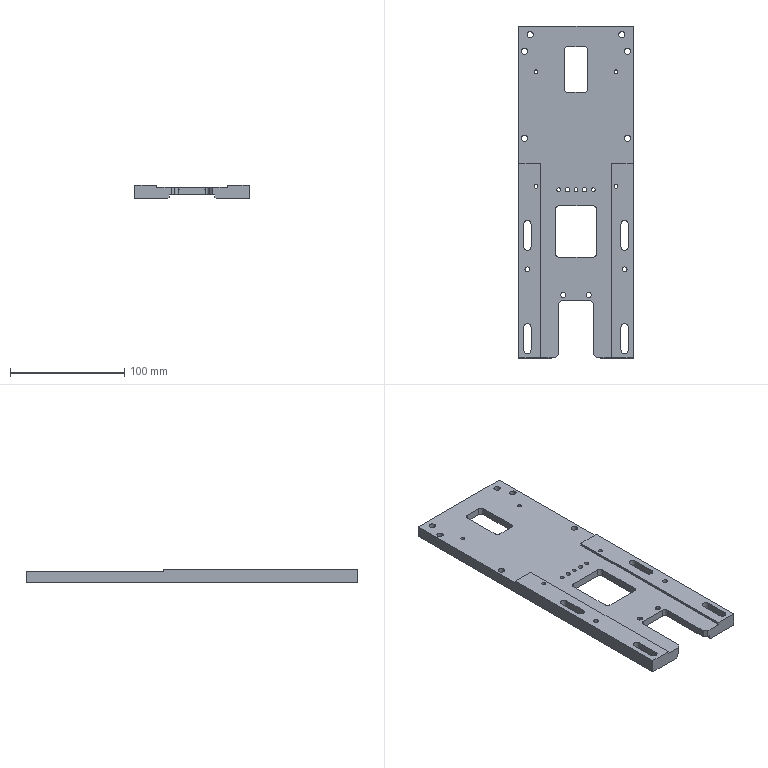Part | SolidWorks | features ICE 9, HoleWzd 5, Chamfer 2, LPattern 2, 3DProfileFeature 1, Extrusion 1, Fillet 1 | 1 solid | 102 faces | box 100 x 290 x 12 mm | volume 225804 mm3 | cylinder 60 | plane 42 | commonest cylinder face diameters 3.3 x14 5.5 x12 6 x10 6.5 x8 4 x4 4.2 x4